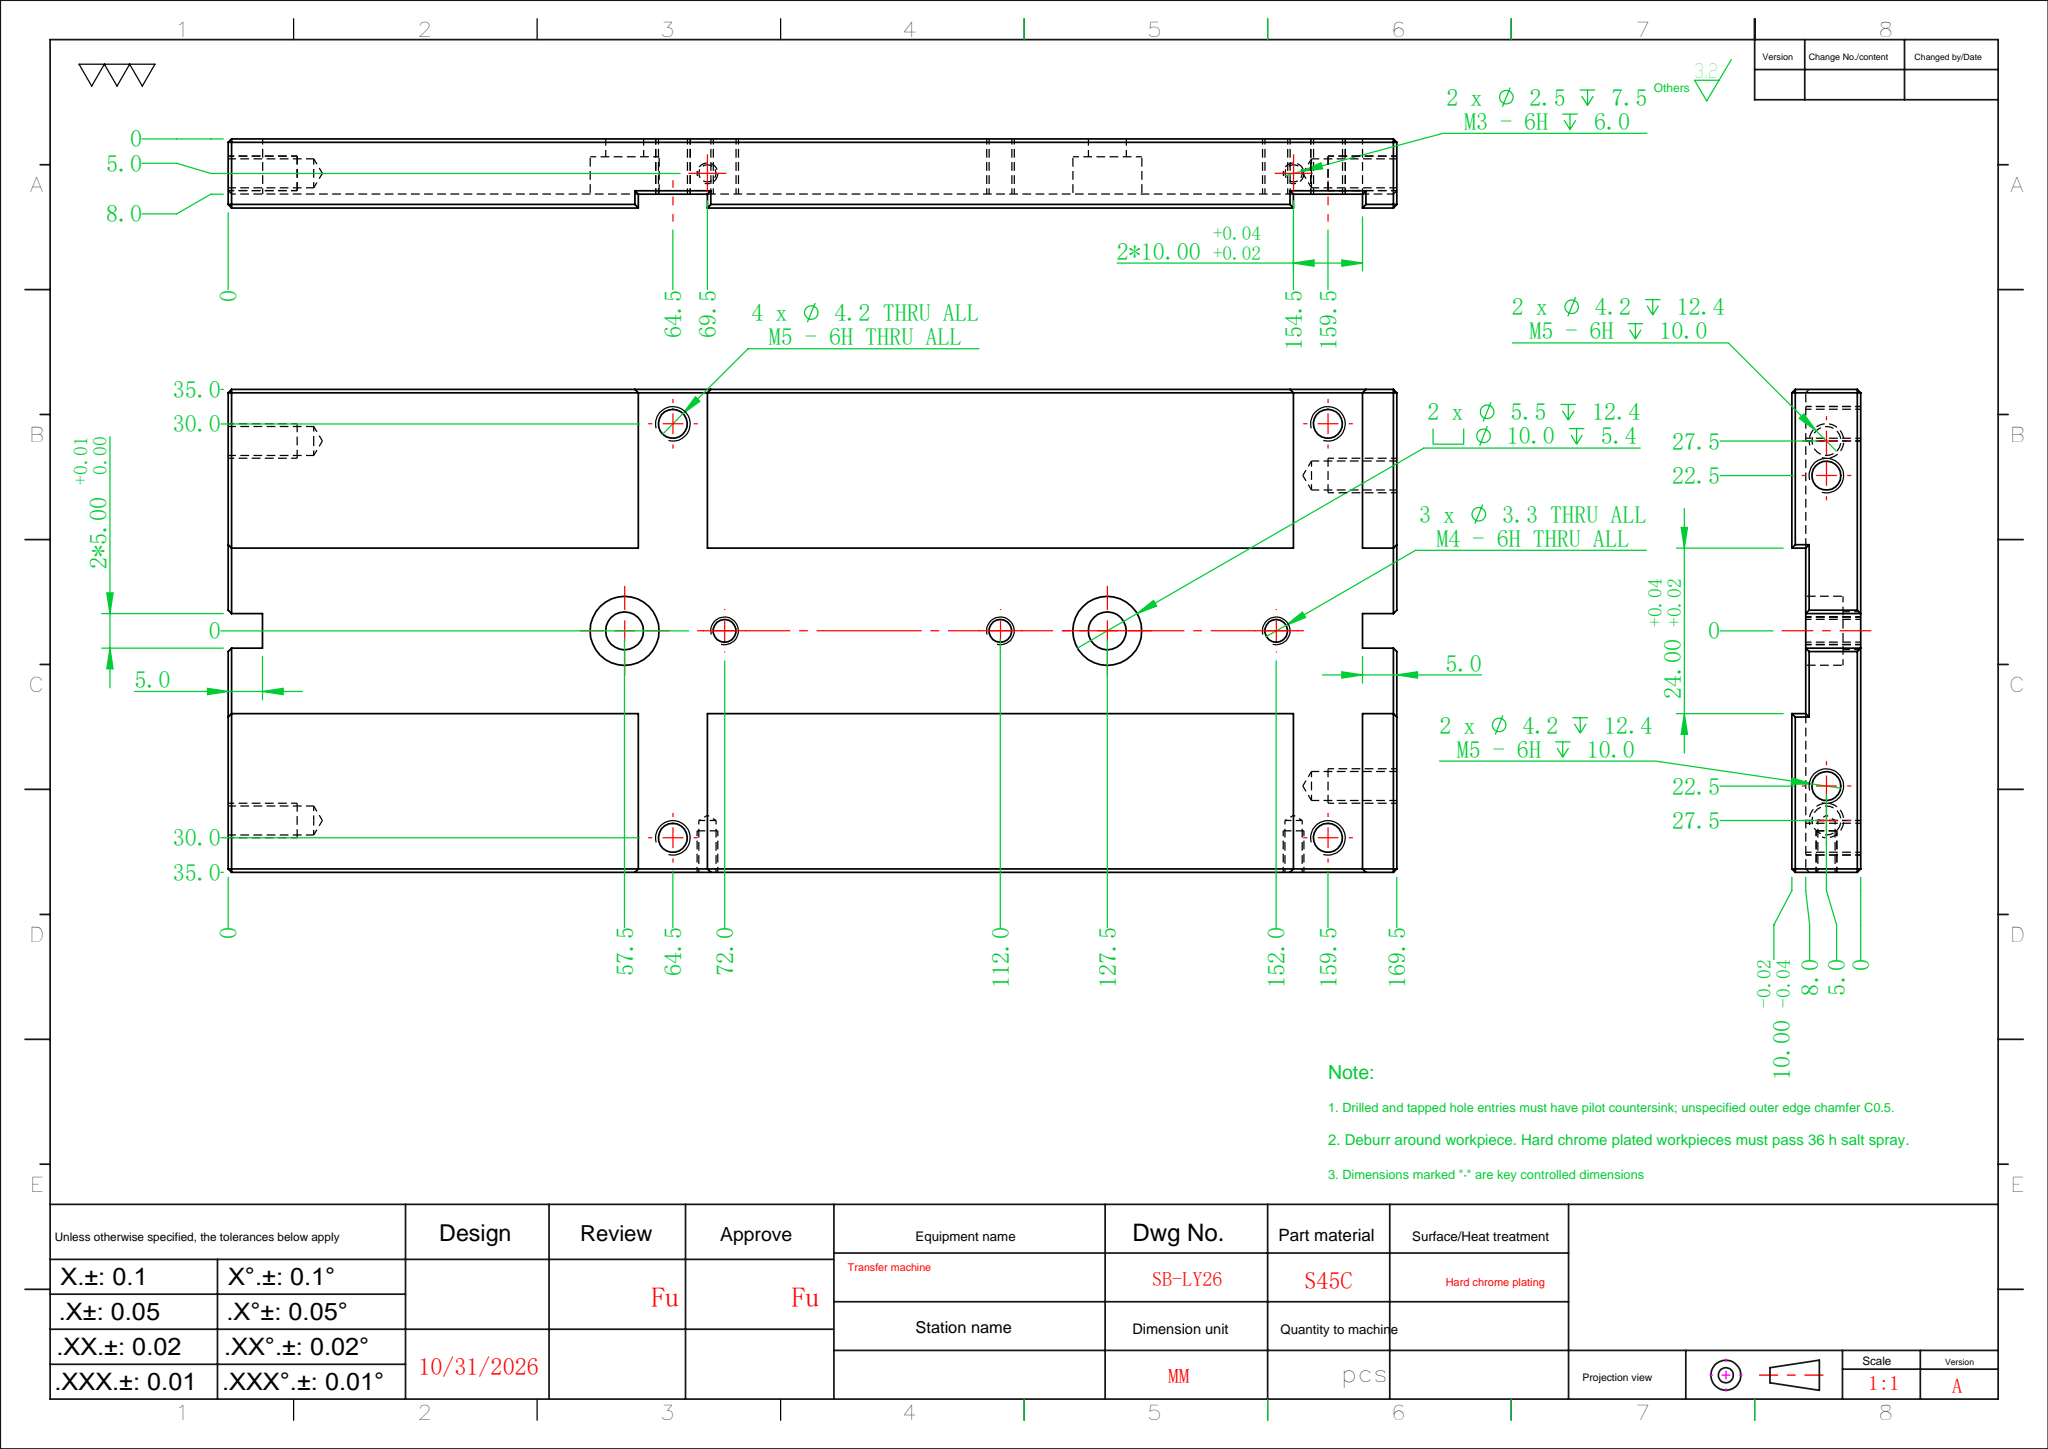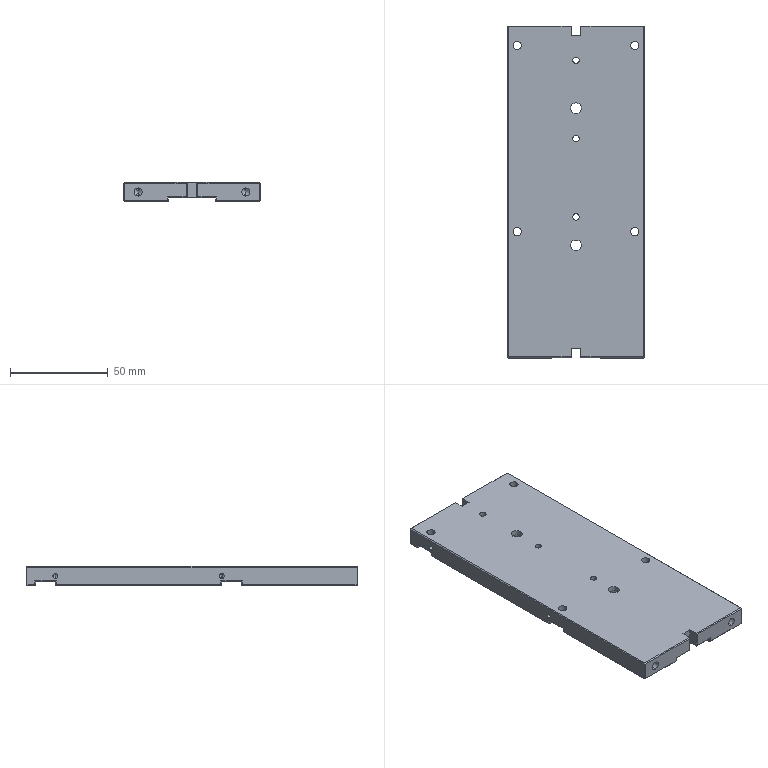Part | SolidWorks | features HoleWzd 6, Cut 4, Chamfer 1, Extrusion 1, ICE 1 | 1 solid | 134 faces | box 70 x 169.5 x 10 mm | volume 105739 mm3 | plane 88 | cylinder 34 | cone 12 | commonest cylinder face diameters 4.2 x16 3.3 x6 2.5 x4 5.5 x4 10 x4